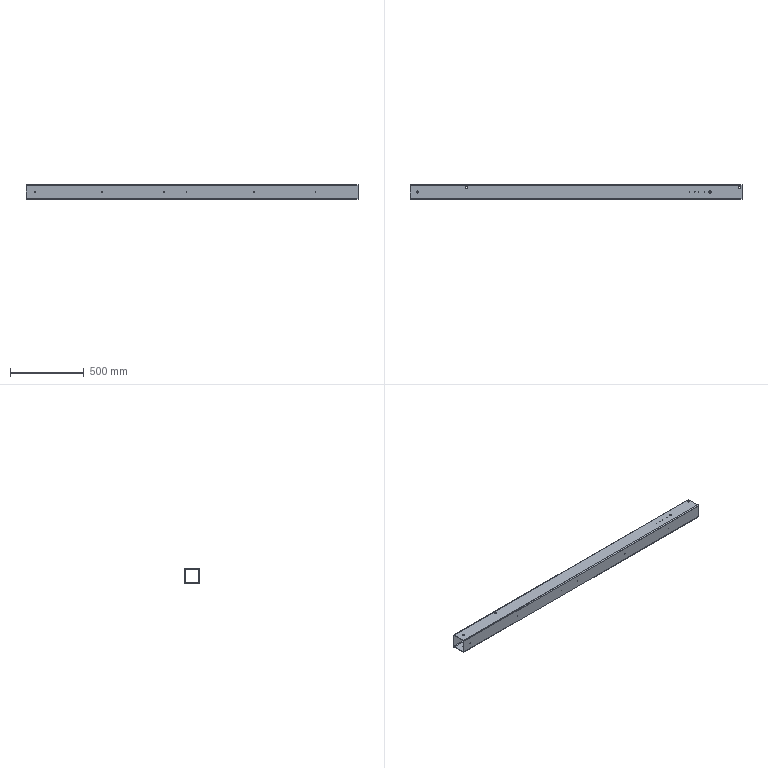Part | STEP file | [05] | 1 solid | 56 faces | box 2252 x 100 x 100 mm | volume 2725742 mm3 | cylinder 46 | plane 10 | commonest cylinder face diameters 15 x16 4 x12 2.5 x8 6.4 x4 12.8 x4 12 x2